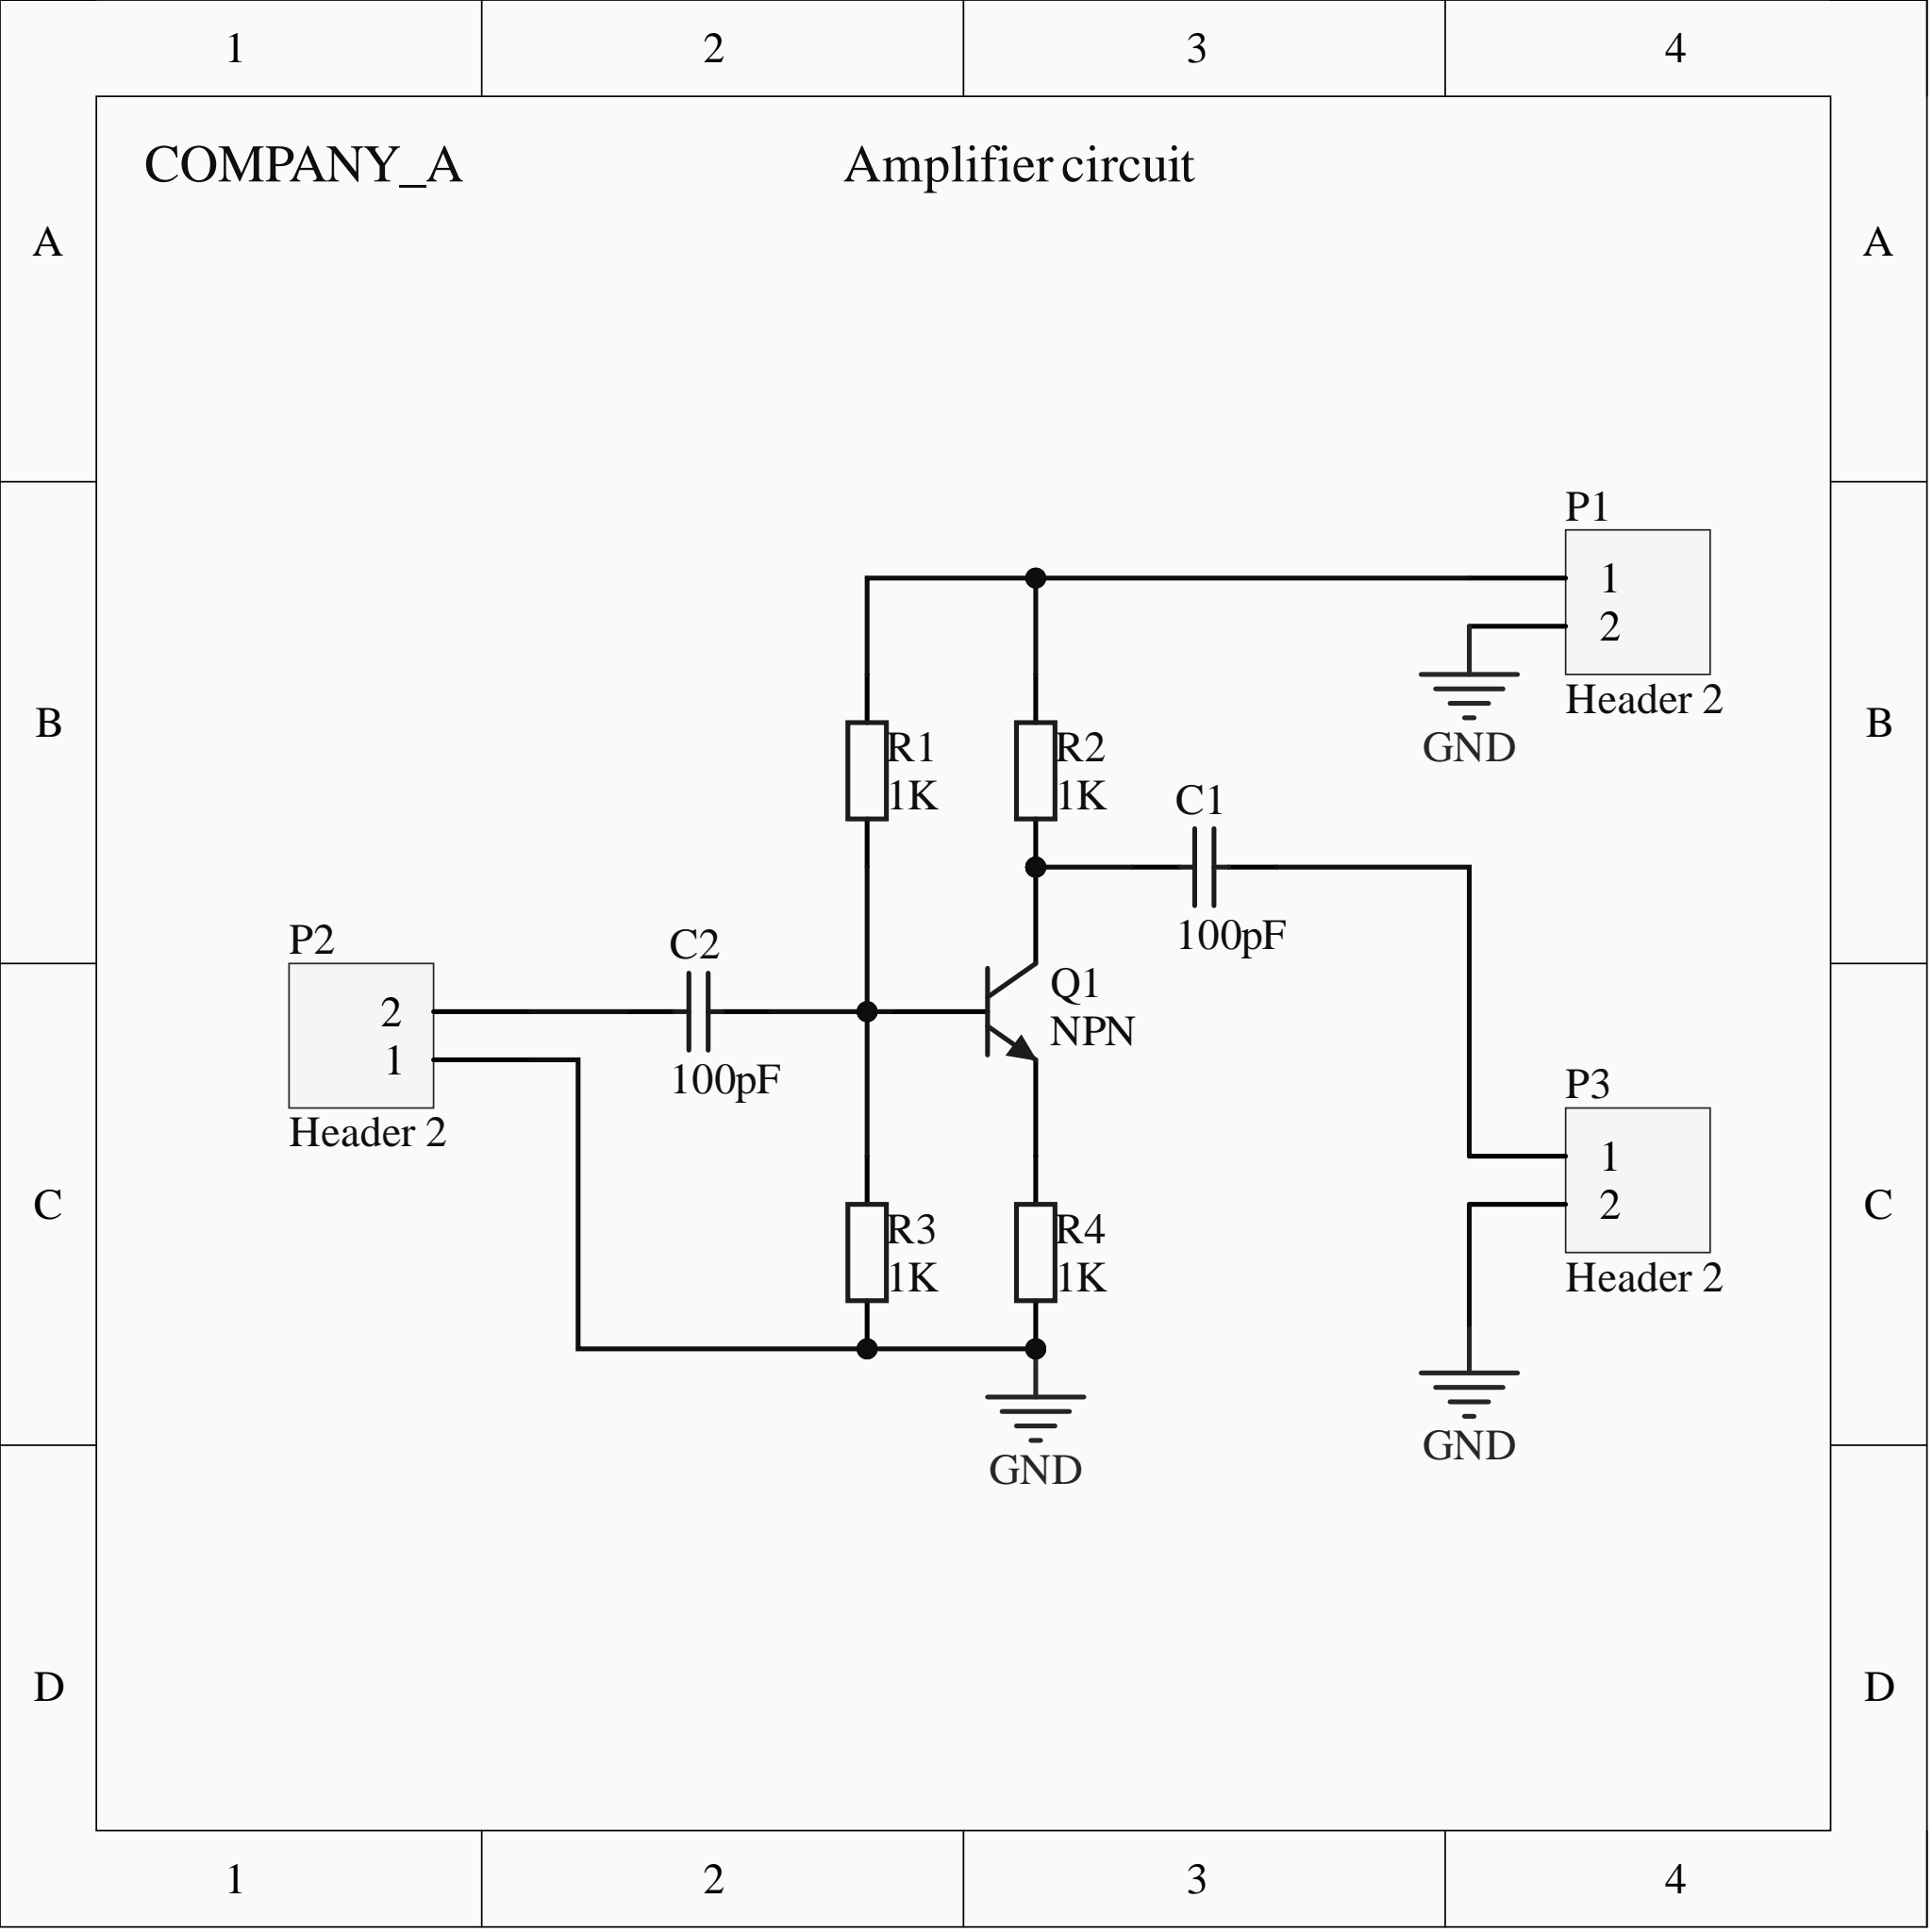Circuit board | Altium Designer | 10 parts | 7 nets
Bill of materials:
Comment,Description,Designator,Footprint,LibRef,Quantity
"100pF","Capacitor","C1, C2","RAD-0.3","Cap","2"
"Header 2","Header, 2-Pin","P1, P2, P3","HDR1X2","Header 2","3"
"NPN","NPN Bipolar Transistor","Q1","TO-226-AA","NPN","1"
"1K","Resistor","R1, R2, R3, R4","AXIAL-0.4","Res2","4"
Netlist (Protel format):
[
C1
RAD-0.3
100pF



]
[
C2
RAD-0.3
100pF



]
[
P1
HDR1X2
Header 2



]
[
P2
HDR1X2
Header 2



]
[
P3
HDR1X2
Header 2



]
[
Q1
TO-226-AA
NPN



]
[
R1
AXIAL-0.4
1K



]
[
R2
AXIAL-0.4
1K



]
[
R3
AXIAL-0.4
1K



]
[
R4
AXIAL-0.4
1K



]
(
NetQ1_3
Q1-3
R4-2
)
(
NetP1_1
P1-1
R1-2
R2-2
)
(
NetC2_2
C2-2
Q1-2
R1-1
R3-2
)
(
NetC2_1
C2-1
P2-2
)
(
NetC1_2
C1-2
P3-1
)
(
NetC1_1
C1-1
Q1-1
R2-1
)
(
GND
P1-2
P2-1
P3-2
R3-1
R4-1
)